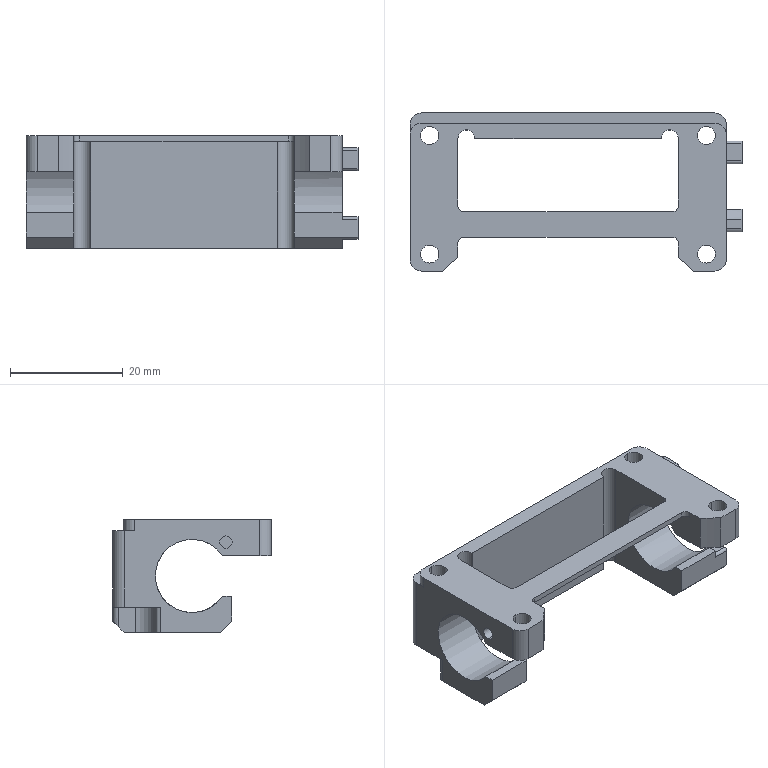NC program | Mastercam | posted with a generic post | part box 58.8 x 28 x 20 mm
Lines 21588 to 23685 of 29451, first 1908 of 2098 lines:
(3 FEM |TOOL - 3|DIA. OFF. - 3|LEN. - 3|TOOL DIA. - 3.)
N3638 T3 M6
N3640 G0 G54 G90 X19.135 Y5.752 C0. B0. S6000 M3
N3642 G43 H3 Z25.
N3644 Z1.
N3646 G1 Z-.25 F600.
N3648 X19.285 F2000.
N3650 G3 X19.435 Y5.902 J.15
N3652 G1 Y9.5
N3654 G2 X17.935 Y8. I-1.5
N3656 G1 X16.978
N3658 G3 X16.828 Y7.85 J-.15
N3660 G1 Y7.7
N3662 X19.135 Y5.752
N3664 Z-.5 F600.
N3666 X19.285 F2000.
N3668 G3 X19.435 Y5.902 J.15
N3670 G1 Y9.5
N3672 G2 X17.935 Y8. I-1.5
N3674 G1 X16.978
N3676 G3 X16.828 Y7.85 J-.15
N3678 G1 Y7.7
N3680 X19.135 Y5.752
N3682 Z-.75 F600.
N3684 X19.285 F2000.
N3686 G3 X19.435 Y5.902 J.15
N3688 G1 Y9.5
N3690 G2 X17.935 Y8. I-1.5
N3692 G1 X16.978
N3694 G3 X16.828 Y7.85 J-.15
N3696 G1 Y7.7
N3698 X19.135 Y5.752
N3700 Z-1. F600.
N3702 X19.285 F2000.
N3704 G3 X19.435 Y5.902 J.15
N3706 G1 Y9.5
N3708 G2 X17.935 Y8. I-1.5
N3710 G1 X16.978
N3712 G3 X16.828 Y7.85 J-.15
N3714 G1 Y7.7
N3716 X19.135 Y5.752
N3718 Z-1.25 F600.
N3720 X19.285 F2000.
N3722 G3 X19.435 Y5.902 J.15
N3724 G1 Y9.5
N3726 G2 X17.935 Y8. I-1.5
N3728 G1 X16.978
N3730 G3 X16.828 Y7.85 J-.15
N3732 G1 Y7.7
N3734 X19.135 Y5.752
N3736 Z-1.5 F600.
N3738 X19.285 F2000.
N3740 G3 X19.435 Y5.902 J.15
N3742 G1 Y9.5
N3744 G2 X17.935 Y8. I-1.5
N3746 G1 X16.978
N3748 G3 X16.828 Y7.85 J-.15
N3750 G1 Y7.7
N3752 X19.135 Y5.752
N3754 Z-1.75 F600.
N3756 X19.285 F2000.
N3758 G3 X19.435 Y5.902 J.15
N3760 G1 Y9.5
N3762 G2 X17.935 Y8. I-1.5
N3764 G1 X16.978
N3766 G3 X16.828 Y7.85 J-.15
N3768 G1 Y7.7
N3770 X19.135 Y5.752
N3772 Z-2. F600.
N3774 X19.285 F2000.
N3776 G3 X19.435 Y5.902 J.15
N3778 G1 Y9.5
N3780 G2 X17.935 Y8. I-1.5
N3782 G1 X16.978
N3784 G3 X16.828 Y7.85 J-.15
N3786 G1 Y7.7
N3788 X19.135 Y5.752
N3790 Z-2.25 F600.
N3792 X19.285 F2000.
N3794 G3 X19.435 Y5.902 J.15
N3796 G1 Y9.5
N3798 G2 X17.935 Y8. I-1.5
N3800 G1 X16.978
N3802 G3 X16.828 Y7.85 J-.15
N3804 G1 Y7.7
N3806 X19.135 Y5.752
N3808 Z-2.5 F600.
N3810 X19.285 F2000.
N3812 G3 X19.435 Y5.902 J.15
N3814 G1 Y9.5
N3816 G2 X17.935 Y8. I-1.5
N3818 G1 X16.978
N3820 G3 X16.828 Y7.85 J-.15
N3822 G1 Y7.7
N3824 X19.135 Y5.752
N3826 Z-2.75 F600.
N3828 X19.285 F2000.
N3830 G3 X19.435 Y5.902 J.15
N3832 G1 Y9.5
N3834 G2 X17.935 Y8. I-1.5
N3836 G1 X16.978
N3838 G3 X16.828 Y7.85 J-.15
N3840 G1 Y7.7
N3842 X19.135 Y5.752
N3844 Z-3. F600.
N3846 X19.285 F2000.
N3848 G3 X19.435 Y5.902 J.15
N3850 G1 Y9.5
N3852 G2 X17.935 Y8. I-1.5
N3854 G1 X16.978
N3856 G3 X16.828 Y7.85 J-.15
N3858 G1 Y7.7
N3860 X19.135 Y5.752
N3862 Z-3.25 F600.
N3864 X19.285 F2000.
N3866 G3 X19.435 Y5.902 J.15
N3868 G1 Y9.5
N3870 G2 X17.935 Y8. I-1.5
N3872 G1 X16.978
N3874 G3 X16.828 Y7.85 J-.15
N3876 G1 Y7.7
N3878 X19.135 Y5.752
N3880 Z-3.5 F600.
N3882 X19.285 F2000.
N3884 G3 X19.435 Y5.902 J.15
N3886 G1 Y9.5
N3888 G2 X17.935 Y8. I-1.5
N3890 G1 X16.978
N3892 G3 X16.828 Y7.85 J-.15
N3894 G1 Y7.7
N3896 X19.135 Y5.752
N3898 Z-3.75 F600.
N3900 X19.285 F2000.
N3902 G3 X19.435 Y5.902 J.15
N3904 G1 Y9.5
N3906 G2 X17.935 Y8. I-1.5
N3908 G1 X16.978
N3910 G3 X16.828 Y7.85 J-.15
N3912 G1 Y7.7
N3914 X19.135 Y5.752
N3916 Z-4. F600.
N3918 X19.285 F2000.
N3920 G3 X19.435 Y5.902 J.15
N3922 G1 Y9.5
N3924 G2 X17.935 Y8. I-1.5
N3926 G1 X16.978
N3928 G3 X16.828 Y7.85 J-.15
N3930 G1 Y7.7
N3932 X19.135 Y5.752
N3934 Z-4.25 F600.
N3936 X19.285 F2000.
N3938 G3 X19.435 Y5.902 J.15
N3940 G1 Y9.5
N3942 G2 X17.935 Y8. I-1.5
N3944 G1 X16.978
N3946 G3 X16.828 Y7.85 J-.15
N3948 G1 Y7.7
N3950 X19.135 Y5.752
N3952 Z-4.5 F600.
N3954 X19.285 F2000.
N3956 G3 X19.435 Y5.902 J.15
N3958 G1 Y9.5
N3960 G2 X17.935 Y8. I-1.5
N3962 G1 X16.978
N3964 G3 X16.828 Y7.85 J-.15
N3966 G1 Y7.7
N3968 X19.135 Y5.752
N3970 Z-4.75 F600.
N3972 X19.285 F2000.
N3974 G3 X19.435 Y5.902 J.15
N3976 G1 Y9.5
N3978 G2 X17.935 Y8. I-1.5
N3980 G1 X16.978
N3982 G3 X16.828 Y7.85 J-.15
N3984 G1 Y7.7
N3986 X19.135 Y5.752
N3988 Z-5. F600.
N3990 X19.285 F2000.
N3992 G3 X19.435 Y5.902 J.15
N3994 G1 Y9.5
N3996 G2 X17.935 Y8. I-1.5
N3998 G1 X16.978
N4000 G3 X16.828 Y7.85 J-.15
N4002 G1 Y7.7
N4004 X19.135 Y5.752
N4006 Z-5.25 F600.
N4008 X19.285 F2000.
N4010 G3 X19.435 Y5.902 J.15
N4012 G1 Y9.5
N4014 G2 X17.935 Y8. I-1.5
N4016 G1 X16.978
N4018 G3 X16.828 Y7.85 J-.15
N4020 G1 Y7.7
N4022 X19.135 Y5.752
N4024 Z-5.5 F600.
N4026 X19.285 F2000.
N4028 G3 X19.435 Y5.902 J.15
N4030 G1 Y9.5
N4032 G2 X17.935 Y8. I-1.5
N4034 G1 X16.978
N4036 G3 X16.828 Y7.85 J-.15
N4038 G1 Y7.7
N4040 X19.135 Y5.752
N4042 Z-5.75 F600.
N4044 X19.285 F2000.
N4046 G3 X19.435 Y5.902 J.15
N4048 G1 Y9.5
N4050 G2 X17.935 Y8. I-1.5
N4052 G1 X16.978
N4054 G3 X16.828 Y7.85 J-.15
N4056 G1 Y7.7
N4058 X19.135 Y5.752
N4060 Z-6. F600.
N4062 X19.285 F2000.
N4064 G3 X19.435 Y5.902 J.15
N4066 G1 Y9.5
N4068 G2 X17.935 Y8. I-1.5
N4070 G1 X16.978
N4072 G3 X16.828 Y7.85 J-.15
N4074 G1 Y7.7
N4076 X19.135 Y5.752
N4078 Z-6.25 F600.
N4080 X19.285 F2000.
N4082 G3 X19.435 Y5.902 J.15
N4084 G1 Y9.5
N4086 G2 X17.935 Y8. I-1.5
N4088 G1 X16.978
N4090 G3 X16.828 Y7.85 J-.15
N4092 G1 Y7.7
N4094 X19.135 Y5.752
N4096 Z-6.5 F600.
N4098 X19.285 F2000.
N4100 G3 X19.435 Y5.902 J.15
N4102 G1 Y9.5
N4104 G2 X17.935 Y8. I-1.5
N4106 G1 X16.978
N4108 G3 X16.828 Y7.85 J-.15
N4110 G1 Y7.7
N4112 X19.135 Y5.752
N4114 Z-6.75 F600.
N4116 X19.285 F2000.
N4118 G3 X19.435 Y5.902 J.15
N4120 G1 Y9.5
N4122 G2 X17.935 Y8. I-1.5
N4124 G1 X16.978
N4126 G3 X16.828 Y7.85 J-.15
N4128 G1 Y7.7
N4130 X19.135 Y5.752
N4132 Z-7. F600.
N4134 X19.285 F2000.
N4136 G3 X19.435 Y5.902 J.15
N4138 G1 Y9.5
N4140 G2 X17.935 Y8. I-1.5
N4142 G1 X16.978
N4144 G3 X16.828 Y7.85 J-.15
N4146 G1 Y7.7
N4148 X19.135 Y5.752
N4150 Z-7.25 F600.
N4152 X19.285 F2000.
N4154 G3 X19.435 Y5.902 J.15
N4156 G1 Y9.5
N4158 G2 X17.935 Y8. I-1.5
N4160 G1 X16.978
N4162 G3 X16.828 Y7.85 J-.15
N4164 G1 Y7.7
N4166 X19.135 Y5.752
N4168 Z-7.5 F600.
N4170 X19.285 F2000.
N4172 G3 X19.435 Y5.902 J.15
N4174 G1 Y9.5
N4176 G2 X17.935 Y8. I-1.5
N4178 G1 X16.978
N4180 G3 X16.828 Y7.85 J-.15
N4182 G1 Y7.7
N4184 X19.135 Y5.752
N4186 Z-7.75 F600.
N4188 X19.285 F2000.
N4190 G3 X19.435 Y5.902 J.15
N4192 G1 Y9.5
N4194 G2 X17.935 Y8. I-1.5
N4196 G1 X16.978
N4198 G3 X16.828 Y7.85 J-.15
N4200 G1 Y7.7
N4202 X19.135 Y5.752
N4204 Z-8. F600.
N4206 X19.285 F2000.
N4208 G3 X19.435 Y5.902 J.15
N4210 G1 Y9.5
N4212 G2 X17.935 Y8. I-1.5
N4214 G1 X16.978
N4216 G3 X16.828 Y7.85 J-.15
N4218 G1 Y7.7
N4220 X19.135 Y5.752
N4222 Z-8.25 F600.
N4224 X19.285 F2000.
N4226 G3 X19.435 Y5.902 J.15
N4228 G1 Y9.5
N4230 G2 X17.935 Y8. I-1.5
N4232 G1 X16.978
N4234 G3 X16.828 Y7.85 J-.15
N4236 G1 Y7.7
N4238 X19.135 Y5.752
N4240 Z-8.5 F600.
N4242 X19.285 F2000.
N4244 G3 X19.435 Y5.902 J.15
N4246 G1 Y9.5
N4248 G2 X17.935 Y8. I-1.5
N4250 G1 X16.978
N4252 G3 X16.828 Y7.85 J-.15
N4254 G1 Y7.7
N4256 X19.135 Y5.752
N4258 Z-8.75 F600.
N4260 X19.285 F2000.
N4262 G3 X19.435 Y5.902 J.15
N4264 G1 Y9.5
N4266 G2 X17.935 Y8. I-1.5
N4268 G1 X16.978
N4270 G3 X16.828 Y7.85 J-.15
N4272 G1 Y7.7
N4274 X19.135 Y5.752
N4276 Z-9. F600.
N4278 X19.285 F2000.
N4280 G3 X19.435 Y5.902 J.15
N4282 G1 Y9.5
N4284 G2 X17.935 Y8. I-1.5
N4286 G1 X16.978
N4288 G3 X16.828 Y7.85 J-.15
N4290 G1 Y7.7
N4292 X19.135 Y5.752
N4294 Z-9.25 F600.
N4296 X19.285 F2000.
N4298 G3 X19.435 Y5.902 J.15
N4300 G1 Y9.5
N4302 G2 X17.935 Y8. I-1.5
N4304 G1 X16.978
N4306 G3 X16.828 Y7.85 J-.15
N4308 G1 Y7.7
N4310 X19.135 Y5.752
N4312 Z-9.5 F600.
N4314 X19.285 F2000.
N4316 G3 X19.435 Y5.902 J.15
N4318 G1 Y9.5
N4320 G2 X17.935 Y8. I-1.5
N4322 G1 X16.978
N4324 G3 X16.828 Y7.85 J-.15
N4326 G1 Y7.7
N4328 X19.135 Y5.752
N4330 Z-9.75 F600.
N4332 X19.285 F2000.
N4334 G3 X19.435 Y5.902 J.15
N4336 G1 Y9.5
N4338 G2 X17.935 Y8. I-1.5
N4340 G1 X16.978
N4342 G3 X16.828 Y7.85 J-.15
N4344 G1 Y7.7
N4346 X19.135 Y5.752
N4348 Z-10. F600.
N4350 X19.285 F2000.
N4352 G3 X19.435 Y5.902 J.15
N4354 G1 Y9.5
N4356 G2 X17.935 Y8. I-1.5
N4358 G1 X16.978
N4360 G3 X16.828 Y7.85 J-.15
N4362 G1 Y7.7
N4364 X19.135 Y5.752
N4366 Z-10.25 F600.
N4368 X19.285 F2000.
N4370 G3 X19.435 Y5.902 J.15
N4372 G1 Y9.5
N4374 G2 X17.935 Y8. I-1.5
N4376 G1 X16.978
N4378 G3 X16.828 Y7.85 J-.15
N4380 G1 Y7.7
N4382 X19.135 Y5.752
N4384 Z-10.5 F600.
N4386 X19.285 F2000.
N4388 G3 X19.435 Y5.902 J.15
N4390 G1 Y9.5
N4392 G2 X17.935 Y8. I-1.5
N4394 G1 X16.978
N4396 G3 X16.828 Y7.85 J-.15
N4398 G1 Y7.7
N4400 X19.135 Y5.752
N4402 Z-10.75 F600.
N4404 X19.285 F2000.
N4406 G3 X19.435 Y5.902 J.15
N4408 G1 Y9.5
N4410 G2 X17.935 Y8. I-1.5
N4412 G1 X16.978
N4414 G3 X16.828 Y7.85 J-.15
N4416 G1 Y7.7
N4418 X19.135 Y5.752
N4420 Z-11. F600.
N4422 X19.285 F2000.
N4424 G3 X19.435 Y5.902 J.15
N4426 G1 Y9.5
N4428 G2 X17.935 Y8. I-1.5
N4430 G1 X16.978
N4432 G3 X16.828 Y7.85 J-.15
N4434 G1 Y7.7
N4436 X19.135 Y5.752
N4438 Z-11.25 F600.
N4440 X19.285 F2000.
N4442 G3 X19.435 Y5.902 J.15
N4444 G1 Y9.5
N4446 G2 X17.935 Y8. I-1.5
N4448 G1 X16.978
N4450 G3 X16.828 Y7.85 J-.15
N4452 G1 Y7.7
N4454 X19.135 Y5.752
N4456 Z-11.5 F600.
N4458 X19.285 F2000.
N4460 G3 X19.435 Y5.902 J.15
N4462 G1 Y9.5
N4464 G2 X17.935 Y8. I-1.5
N4466 G1 X16.978
N4468 G3 X16.828 Y7.85 J-.15
N4470 G1 Y7.7
N4472 X19.135 Y5.752
N4474 Z-11.75 F600.
N4476 X19.285 F2000.
N4478 G3 X19.435 Y5.902 J.15
N4480 G1 Y9.5
N4482 G2 X17.935 Y8. I-1.5
N4484 G1 X16.978
N4486 G3 X16.828 Y7.85 J-.15
N4488 G1 Y7.7
N4490 X19.135 Y5.752
N4492 Z-12. F600.
N4494 X19.285 F2000.
N4496 G3 X19.435 Y5.902 J.15
N4498 G1 Y9.5
N4500 G2 X17.935 Y8. I-1.5
N4502 G1 X16.978
N4504 G3 X16.828 Y7.85 J-.15
N4506 G1 Y7.7
N4508 X19.135 Y5.752
N4510 Z-12.25 F600.
N4512 X19.285 F2000.
N4514 G3 X19.435 Y5.902 J.15
N4516 G1 Y9.5
N4518 G2 X17.935 Y8. I-1.5
N4520 G1 X16.978
N4522 G3 X16.828 Y7.85 J-.15
N4524 G1 Y7.7
N4526 X19.135 Y5.752
N4528 Z-12.5 F600.
N4530 X19.285 F2000.
N4532 G3 X19.435 Y5.902 J.15
N4534 G1 Y9.5
N4536 G2 X17.935 Y8. I-1.5
N4538 G1 X16.978
N4540 G3 X16.828 Y7.85 J-.15
N4542 G1 Y7.7
N4544 X19.135 Y5.752
N4546 Z-12.75 F600.
N4548 X19.285 F2000.
N4550 G3 X19.435 Y5.902 J.15
N4552 G1 Y9.5
N4554 G2 X17.935 Y8. I-1.5
N4556 G1 X16.978
N4558 G3 X16.828 Y7.85 J-.15
N4560 G1 Y7.7
N4562 X19.135 Y5.752
N4564 Z-13. F600.
N4566 X19.285 F2000.
N4568 G3 X19.435 Y5.902 J.15
N4570 G1 Y9.5
N4572 G2 X17.935 Y8. I-1.5
N4574 G1 X16.978
N4576 G3 X16.828 Y7.85 J-.15
N4578 G1 Y7.7
N4580 X19.135 Y5.752
N4582 Z-13.25 F600.
N4584 X19.285 F2000.
N4586 G3 X19.435 Y5.902 J.15
N4588 G1 Y9.5
N4590 G2 X17.935 Y8. I-1.5
N4592 G1 X16.978
N4594 G3 X16.828 Y7.85 J-.15
N4596 G1 Y7.7
N4598 X19.135 Y5.752
N4600 Z-13.5 F600.
N4602 X19.285 F2000.
N4604 G3 X19.435 Y5.902 J.15
N4606 G1 Y9.5
N4608 G2 X17.935 Y8. I-1.5
N4610 G1 X16.978
N4612 G3 X16.828 Y7.85 J-.15
N4614 G1 Y7.7
N4616 X19.135 Y5.752
N4618 Z-13.75 F600.
N4620 X19.285 F2000.
N4622 G3 X19.435 Y5.902 J.15
N4624 G1 Y9.5
N4626 G2 X17.935 Y8. I-1.5
N4628 G1 X16.978
N4630 G3 X16.828 Y7.85 J-.15
N4632 G1 Y7.7
N4634 X19.135 Y5.752
N4636 Z-14. F600.
N4638 X19.285 F2000.
N4640 G3 X19.435 Y5.902 J.15
N4642 G1 Y9.5
N4644 G2 X17.935 Y8. I-1.5
N4646 G1 X16.978
N4648 G3 X16.828 Y7.85 J-.15
N4650 G1 Y7.7
N4652 X19.135 Y5.752
N4654 Z-14.25 F600.
N4656 X19.285 F2000.
N4658 G3 X19.435 Y5.902 J.15
N4660 G1 Y9.5
N4662 G2 X17.935 Y8. I-1.5
N4664 G1 X16.978
N4666 G3 X16.828 Y7.85 J-.15
N4668 G1 Y7.7
N4670 X19.135 Y5.752
N4672 Z-14.5 F600.
N4674 X19.285 F2000.
N4676 G3 X19.435 Y5.902 J.15
N4678 G1 Y9.5
N4680 G2 X17.935 Y8. I-1.5
N4682 G1 X16.978
N4684 G3 X16.828 Y7.85 J-.15
N4686 G1 Y7.7
N4688 X19.135 Y5.752
N4690 Z-14.75 F600.
N4692 X19.285 F2000.
N4694 G3 X19.435 Y5.902 J.15
N4696 G1 Y9.5
N4698 G2 X17.935 Y8. I-1.5
N4700 G1 X16.978
N4702 G3 X16.828 Y7.85 J-.15
N4704 G1 Y7.7
N4706 X19.135 Y5.752
N4708 Z-15. F600.
N4710 X19.285 F2000.
N4712 G3 X19.435 Y5.902 J.15
N4714 G1 Y9.5
N4716 G2 X17.935 Y8. I-1.5
N4718 G1 X16.978
N4720 G3 X16.828 Y7.85 J-.15
N4722 G1 Y7.7
N4724 X19.135 Y5.752
N4726 Z-15.25 F600.
N4728 X19.285 F2000.
N4730 G3 X19.435 Y5.902 J.15
N4732 G1 Y9.5
N4734 G2 X17.935 Y8. I-1.5
N4736 G1 X16.978
N4738 G3 X16.828 Y7.85 J-.15
N4740 G1 Y7.7
N4742 X19.135 Y5.752
N4744 Z-15.5 F600.
N4746 X19.285 F2000.
N4748 G3 X19.435 Y5.902 J.15
N4750 G1 Y9.5
N4752 G2 X17.935 Y8. I-1.5
N4754 G1 X16.978
N4756 G3 X16.828 Y7.85 J-.15
N4758 G1 Y7.7
N4760 X19.135 Y5.752
N4762 Z-15.75 F600.
N4764 X19.285 F2000.
N4766 G3 X19.435 Y5.902 J.15
N4768 G1 Y9.5
N4770 G2 X17.935 Y8. I-1.5
N4772 G1 X16.978
N4774 G3 X16.828 Y7.85 J-.15
N4776 G1 Y7.7
N4778 X19.135 Y5.752
N4780 Z-16. F600.
N4782 X19.285 F2000.
N4784 G3 X19.435 Y5.902 J.15
N4786 G1 Y9.5
N4788 G2 X17.935 Y8. I-1.5
N4790 G1 X16.978
N4792 G3 X16.828 Y7.85 J-.15
N4794 G1 Y7.7
N4796 X19.135 Y5.752
N4798 Z-16.25 F600.
N4800 X19.285 F2000.
N4802 G3 X19.435 Y5.902 J.15
N4804 G1 Y9.5
N4806 G2 X17.935 Y8. I-1.5
N4808 G1 X16.978
N4810 G3 X16.828 Y7.85 J-.15
N4812 G1 Y7.7
N4814 X19.135 Y5.752
N4816 Z-16.5 F600.
N4818 X19.285 F2000.
N4820 G3 X19.435 Y5.902 J.15
N4822 G1 Y9.5
N4824 G2 X17.935 Y8. I-1.5
N4826 G1 X16.978
N4828 G3 X16.828 Y7.85 J-.15
N4830 G1 Y7.7
N4832 X19.135 Y5.752
N4834 Z-16.75 F600.
N4836 X19.285 F2000.
N4838 G3 X19.435 Y5.902 J.15
N4840 G1 Y9.5
N4842 G2 X17.935 Y8. I-1.5
N4844 G1 X16.978
N4846 G3 X16.828 Y7.85 J-.15
N4848 G1 Y7.7
N4850 X19.135 Y5.752
N4852 Z-17. F600.
N4854 X19.285 F2000.
N4856 G3 X19.435 Y5.902 J.15
N4858 G1 Y9.5
N4860 G2 X17.935 Y8. I-1.5
N4862 G1 X16.978
N4864 G3 X16.828 Y7.85 J-.15
N4866 G1 Y7.7
N4868 X19.135 Y5.752
N4870 Z-17.25 F600.
N4872 X19.285 F2000.
N4874 G3 X19.435 Y5.902 J.15
N4876 G1 Y9.5
N4878 G2 X17.935 Y8. I-1.5
N4880 G1 X16.978
N4882 G3 X16.828 Y7.85 J-.15
N4884 G1 Y7.7
N4886 X19.135 Y5.752
N4888 Z-17.5 F600.
N4890 X19.285 F2000.
N4892 G3 X19.435 Y5.902 J.15
N4894 G1 Y9.5
N4896 G2 X17.935 Y8. I-1.5
N4898 G1 X16.978
N4900 G3 X16.828 Y7.85 J-.15
N4902 G1 Y7.7
N4904 X19.135 Y5.752
N4906 Z-17.75 F600.
N4908 X19.285 F2000.
N4910 G3 X19.435 Y5.902 J.15
N4912 G1 Y9.5
N4914 G2 X17.935 Y8. I-1.5
N4916 G1 X16.978
N4918 G3 X16.828 Y7.85 J-.15
N4920 G1 Y7.7
N4922 X19.135 Y5.752
N4924 Z-18. F600.
N4926 X19.285 F2000.
N4928 G3 X19.435 Y5.902 J.15
N4930 G1 Y9.5
N4932 G2 X17.935 Y8. I-1.5
N4934 G1 X16.978
N4936 G3 X16.828 Y7.85 J-.15
N4938 G1 Y7.7
N4940 X19.135 Y5.752
N4942 Z-18.25 F600.
N4944 X19.285 F2000.
N4946 G3 X19.435 Y5.902 J.15
N4948 G1 Y9.5
N4950 G2 X17.935 Y8. I-1.5
N4952 G1 X16.978
N4954 G3 X16.828 Y7.85 J-.15
N4956 G1 Y7.7
N4958 X19.135 Y5.752
N4960 Z-18.5 F600.
N4962 X19.285 F2000.
N4964 G3 X19.435 Y5.902 J.15
N4966 G1 Y9.5
N4968 G2 X17.935 Y8. I-1.5
N4970 G1 X16.978
N4972 G3 X16.828 Y7.85 J-.15
N4974 G1 Y7.7
N4976 X19.135 Y5.752
N4978 Z-18.75 F600.
N4980 X19.285 F2000.
N4982 G3 X19.435 Y5.902 J.15
N4984 G1 Y9.5
N4986 G2 X17.935 Y8. I-1.5
N4988 G1 X16.978
N4990 G3 X16.828 Y7.85 J-.15
N4992 G1 Y7.7
N4994 X19.135 Y5.752
N4996 Z-19. F600.
N4998 X19.285 F2000.
N5000 G3 X19.435 Y5.902 J.15
N5002 G1 Y9.5
N5004 G2 X17.935 Y8. I-1.5
N5006 G1 X16.978
N5008 G3 X16.828 Y7.85 J-.15
N5010 G1 Y7.7
N5012 X19.135 Y5.752
N5014 Z-19.25 F600.
N5016 X19.285 F2000.
N5018 G3 X19.435 Y5.902 J.15
N5020 G1 Y9.5
N5022 G2 X17.935 Y8. I-1.5
N5024 G1 X16.978
N5026 G3 X16.828 Y7.85 J-.15
N5028 G1 Y7.7
N5030 X19.135 Y5.752
N5032 Z-19.5 F600.
N5034 X19.285 F2000.
N5036 G3 X19.435 Y5.902 J.15
N5038 G1 Y9.5
N5040 G2 X17.935 Y8. I-1.5
N5042 G1 X16.978
N5044 G3 X16.828 Y7.85 J-.15
N5046 G1 Y7.7
N5048 X19.135 Y5.752
N5050 Z-19.75 F600.
N5052 X19.285 F2000.
N5054 G3 X19.435 Y5.902 J.15
N5056 G1 Y9.5
N5058 G2 X17.935 Y8. I-1.5
N5060 G1 X16.978
N5062 G3 X16.828 Y7.85 J-.15
N5064 G1 Y7.7
N5066 X19.135 Y5.752
N5068 Z-20. F600.
N5070 X19.285 F2000.
N5072 G3 X19.435 Y5.902 J.15
N5074 G1 Y9.5
N5076 G2 X17.935 Y8. I-1.5
N5078 G1 X16.978
N5080 G3 X16.828 Y7.85 J-.15
N5082 G1 Y7.7
N5084 X19.135 Y5.752
N5086 Z-20.25 F600.
N5088 X19.285 F2000.
N5090 G3 X19.435 Y5.902 J.15
N5092 G1 Y9.5
N5094 G2 X17.935 Y8. I-1.5
N5096 G1 X16.978
N5098 G3 X16.828 Y7.85 J-.15
N5100 G1 Y7.7
N5102 X19.135 Y5.752
N5104 Z-20.5 F600.
N5106 X19.285 F2000.
N5108 G3 X19.435 Y5.902 J.15
N5110 G1 Y9.5
N5112 G2 X17.935 Y8. I-1.5
N5114 G1 X16.978
N5116 G3 X16.828 Y7.85 J-.15
N5118 G1 Y7.7
N5120 G0 Z25.
N5122 X-14.028
N5124 Z1.
N5126 G1 Z-.25 F600.
N5128 Y7.85 F2000.
N5130 G3 X-14.178 Y8. I-.15
N5132 G1 X-15.135
N5134 G2 X-16.635 Y9.5 J1.5
N5136 G1 Y5.902
N5138 G3 X-16.485 Y5.752 I.15
N5140 G1 X-16.335
N5142 X-14.028 Y7.7
N5144 Z-.5 F600.
N5146 Y7.85 F2000.
N5148 G3 X-14.178 Y8. I-.15
N5150 G1 X-15.135
N5152 G2 X-16.635 Y9.5 J1.5
N5154 G1 Y5.902
N5156 G3 X-16.485 Y5.752 I.15
N5158 G1 X-16.335
N5160 X-14.028 Y7.7
N5162 Z-.75 F600.
N5164 Y7.85 F2000.
N5166 G3 X-14.178 Y8. I-.15
N5168 G1 X-15.135
N5170 G2 X-16.635 Y9.5 J1.5
N5172 G1 Y5.902
N5174 G3 X-16.485 Y5.752 I.15
N5176 G1 X-16.335
N5178 X-14.028 Y7.7
N5180 Z-1. F600.
N5182 Y7.85 F2000.
N5184 G3 X-14.178 Y8. I-.15
N5186 G1 X-15.135
N5188 G2 X-16.635 Y9.5 J1.5
N5190 G1 Y5.902
N5192 G3 X-16.485 Y5.752 I.15
N5194 G1 X-16.335
N5196 X-14.028 Y7.7
N5198 Z-1.25 F600.
N5200 Y7.85 F2000.
N5202 G3 X-14.178 Y8. I-.15
N5204 G1 X-15.135
N5206 G2 X-16.635 Y9.5 J1.5
N5208 G1 Y5.902
N5210 G3 X-16.485 Y5.752 I.15
N5212 G1 X-16.335
N5214 X-14.028 Y7.7
N5216 Z-1.5 F600.
N5218 Y7.85 F2000.
N5220 G3 X-14.178 Y8. I-.15
N5222 G1 X-15.135
N5224 G2 X-16.635 Y9.5 J1.5
N5226 G1 Y5.902
N5228 G3 X-16.485 Y5.752 I.15
N5230 G1 X-16.335
N5232 X-14.028 Y7.7
N5234 Z-1.75 F600.
N5236 Y7.85 F2000.
N5238 G3 X-14.178 Y8. I-.15
N5240 G1 X-15.135
N5242 G2 X-16.635 Y9.5 J1.5
N5244 G1 Y5.902
N5246 G3 X-16.485 Y5.752 I.15
N5248 G1 X-16.335
N5250 X-14.028 Y7.7
N5252 Z-2. F600.
N5254 Y7.85 F2000.
N5256 G3 X-14.178 Y8. I-.15
N5258 G1 X-15.135
N5260 G2 X-16.635 Y9.5 J1.5
N5262 G1 Y5.902
N5264 G3 X-16.485 Y5.752 I.15
N5266 G1 X-16.335
N5268 X-14.028 Y7.7
N5270 Z-2.25 F600.
N5272 Y7.85 F2000.
N5274 G3 X-14.178 Y8. I-.15
N5276 G1 X-15.135
N5278 G2 X-16.635 Y9.5 J1.5
N5280 G1 Y5.902
N5282 G3 X-16.485 Y5.752 I.15
N5284 G1 X-16.335
N5286 X-14.028 Y7.7
N5288 Z-2.5 F600.
N5290 Y7.85 F2000.
N5292 G3 X-14.178 Y8. I-.15
N5294 G1 X-15.135
N5296 G2 X-16.635 Y9.5 J1.5
N5298 G1 Y5.902
N5300 G3 X-16.485 Y5.752 I.15
N5302 G1 X-16.335
N5304 X-14.028 Y7.7
N5306 Z-2.75 F600.
N5308 Y7.85 F2000.
N5310 G3 X-14.178 Y8. I-.15
N5312 G1 X-15.135
N5314 G2 X-16.635 Y9.5 J1.5
N5316 G1 Y5.902
N5318 G3 X-16.485 Y5.752 I.15
N5320 G1 X-16.335
N5322 X-14.028 Y7.7
N5324 Z-3. F600.
N5326 Y7.85 F2000.
N5328 G3 X-14.178 Y8. I-.15
N5330 G1 X-15.135
N5332 G2 X-16.635 Y9.5 J1.5
N5334 G1 Y5.902
N5336 G3 X-16.485 Y5.752 I.15
N5338 G1 X-16.335
N5340 X-14.028 Y7.7
N5342 Z-3.25 F600.
N5344 Y7.85 F2000.
N5346 G3 X-14.178 Y8. I-.15
N5348 G1 X-15.135
N5350 G2 X-16.635 Y9.5 J1.5
N5352 G1 Y5.902
N5354 G3 X-16.485 Y5.752 I.15
N5356 G1 X-16.335
N5358 X-14.028 Y7.7
N5360 Z-3.5 F600.
N5362 Y7.85 F2000.
N5364 G3 X-14.178 Y8. I-.15
N5366 G1 X-15.135
N5368 G2 X-16.635 Y9.5 J1.5
N5370 G1 Y5.902
N5372 G3 X-16.485 Y5.752 I.15
N5374 G1 X-16.335
N5376 X-14.028 Y7.7
N5378 Z-3.75 F600.
N5380 Y7.85 F2000.
N5382 G3 X-14.178 Y8. I-.15
N5384 G1 X-15.135
N5386 G2 X-16.635 Y9.5 J1.5
N5388 G1 Y5.902
N5390 G3 X-16.485 Y5.752 I.15
N5392 G1 X-16.335
N5394 X-14.028 Y7.7
N5396 Z-4. F600.
N5398 Y7.85 F2000.
N5400 G3 X-14.178 Y8. I-.15
N5402 G1 X-15.135
N5404 G2 X-16.635 Y9.5 J1.5
N5406 G1 Y5.902
N5408 G3 X-16.485 Y5.752 I.15
N5410 G1 X-16.335
N5412 X-14.028 Y7.7
N5414 Z-4.25 F600.
N5416 Y7.85 F2000.
N5418 G3 X-14.178 Y8. I-.15
N5420 G1 X-15.135
N5422 G2 X-16.635 Y9.5 J1.5
N5424 G1 Y5.902
N5426 G3 X-16.485 Y5.752 I.15
N5428 G1 X-16.335
N5430 X-14.028 Y7.7
N5432 Z-4.5 F600.
N5434 Y7.85 F2000.
N5436 G3 X-14.178 Y8. I-.15
N5438 G1 X-15.135
N5440 G2 X-16.635 Y9.5 J1.5
N5442 G1 Y5.902
N5444 G3 X-16.485 Y5.752 I.15
N5446 G1 X-16.335
N5448 X-14.028 Y7.7
N5450 Z-4.75 F600.
N5452 Y7.85 F2000.
N5454 G3 X-14.178 Y8. I-.15
N5456 G1 X-15.135
N5458 G2 X-16.635 Y9.5 J1.5
N5460 G1 Y5.902
N5462 G3 X-16.485 Y5.752 I.15
N5464 G1 X-16.335
N5466 X-14.028 Y7.7
N5468 Z-5. F600.
N5470 Y7.85 F2000.
N5472 G3 X-14.178 Y8. I-.15
N5474 G1 X-15.135
N5476 G2 X-16.635 Y9.5 J1.5
N5478 G1 Y5.902
N5480 G3 X-16.485 Y5.752 I.15
N5482 G1 X-16.335
N5484 X-14.028 Y7.7
N5486 Z-5.25 F600.
N5488 Y7.85 F2000.
N5490 G3 X-14.178 Y8. I-.15
N5492 G1 X-15.135
N5494 G2 X-16.635 Y9.5 J1.5
N5496 G1 Y5.902
N5498 G3 X-16.485 Y5.752 I.15
N5500 G1 X-16.335
N5502 X-14.028 Y7.7
N5504 Z-5.5 F600.
N5506 Y7.85 F2000.
N5508 G3 X-14.178 Y8. I-.15
N5510 G1 X-15.135
N5512 G2 X-16.635 Y9.5 J1.5
N5514 G1 Y5.902
N5516 G3 X-16.485 Y5.752 I.15
N5518 G1 X-16.335
N5520 X-14.028 Y7.7
N5522 Z-5.75 F600.
N5524 Y7.85 F2000.
N5526 G3 X-14.178 Y8. I-.15
N5528 G1 X-15.135
N5530 G2 X-16.635 Y9.5 J1.5
N5532 G1 Y5.902
N5534 G3 X-16.485 Y5.752 I.15
N5536 G1 X-16.335
N5538 X-14.028 Y7.7
N5540 Z-6. F600.
N5542 Y7.85 F2000.
N5544 G3 X-14.178 Y8. I-.15
N5546 G1 X-15.135
N5548 G2 X-16.635 Y9.5 J1.5
N5550 G1 Y5.902
N5552 G3 X-16.485 Y5.752 I.15
N5554 G1 X-16.335
N5556 X-14.028 Y7.7
N5558 Z-6.25 F600.
N5560 Y7.85 F2000.
N5562 G3 X-14.178 Y8. I-.15
N5564 G1 X-15.135
N5566 G2 X-16.635 Y9.5 J1.5
N5568 G1 Y5.902
N5570 G3 X-16.485 Y5.752 I.15
N5572 G1 X-16.335
N5574 X-14.028 Y7.7
N5576 Z-6.5 F600.
N5578 Y7.85 F2000.
N5580 G3 X-14.178 Y8. I-.15
N5582 G1 X-15.135
N5584 G2 X-16.635 Y9.5 J1.5
N5586 G1 Y5.902
N5588 G3 X-16.485 Y5.752 I.15
N5590 G1 X-16.335
N5592 X-14.028 Y7.7
N5594 Z-6.75 F600.
N5596 Y7.85 F2000.
N5598 G3 X-14.178 Y8. I-.15
N5600 G1 X-15.135
N5602 G2 X-16.635 Y9.5 J1.5
N5604 G1 Y5.902
N5606 G3 X-16.485 Y5.752 I.15
N5608 G1 X-16.335
N5610 X-14.028 Y7.7
N5612 Z-7. F600.
N5614 Y7.85 F2000.
N5616 G3 X-14.178 Y8. I-.15
N5618 G1 X-15.135
N5620 G2 X-16.635 Y9.5 J1.5
N5622 G1 Y5.902
N5624 G3 X-16.485 Y5.752 I.15
N5626 G1 X-16.335
N5628 X-14.028 Y7.7
N5630 Z-7.25 F600.
N5632 Y7.85 F2000.
N5634 G3 X-14.178 Y8. I-.15
N5636 G1 X-15.135
N5638 G2 X-16.635 Y9.5 J1.5
N5640 G1 Y5.902
N5642 G3 X-16.485 Y5.752 I.15
N5644 G1 X-16.335
N5646 X-14.028 Y7.7
N5648 Z-7.5 F600.
N5650 Y7.85 F2000.
N5652 G3 X-14.178 Y8. I-.15
N5654 G1 X-15.135
N5656 G2 X-16.635 Y9.5 J1.5
N5658 G1 Y5.902
N5660 G3 X-16.485 Y5.752 I.15
N5662 G1 X-16.335
N5664 X-14.028 Y7.7
N5666 Z-7.75 F600.
N5668 Y7.85 F2000.
N5670 G3 X-14.178 Y8. I-.15
N5672 G1 X-15.135
N5674 G2 X-16.635 Y9.5 J1.5
N5676 G1 Y5.902
N5678 G3 X-16.485 Y5.752 I.15
N5680 G1 X-16.335
N5682 X-14.028 Y7.7
N5684 Z-8. F600.
N5686 Y7.85 F2000.
N5688 G3 X-14.178 Y8. I-.15
N5690 G1 X-15.135
N5692 G2 X-16.635 Y9.5 J1.5
N5694 G1 Y5.902
N5696 G3 X-16.485 Y5.752 I.15
N5698 G1 X-16.335
N5700 X-14.028 Y7.7
N5702 Z-8.25 F600.
N5704 Y7.85 F2000.
N5706 G3 X-14.178 Y8. I-.15
N5708 G1 X-15.135
N5710 G2 X-16.635 Y9.5 J1.5
N5712 G1 Y5.902
N5714 G3 X-16.485 Y5.752 I.15
N5716 G1 X-16.335
N5718 X-14.028 Y7.7
N5720 Z-8.5 F600.
N5722 Y7.85 F2000.
N5724 G3 X-14.178 Y8. I-.15
N5726 G1 X-15.135
N5728 G2 X-16.635 Y9.5 J1.5
N5730 G1 Y5.902
N5732 G3 X-16.485 Y5.752 I.15
N5734 G1 X-16.335
N5736 X-14.028 Y7.7
N5738 Z-8.75 F600.
N5740 Y7.85 F2000.
N5742 G3 X-14.178 Y8. I-.15
N5744 G1 X-15.135
N5746 G2 X-16.635 Y9.5 J1.5
N5748 G1 Y5.902
N5750 G3 X-16.485 Y5.752 I.15
N5752 G1 X-16.335
N5754 X-14.028 Y7.7
N5756 Z-9. F600.
N5758 Y7.85 F2000.
N5760 G3 X-14.178 Y8. I-.15
N5762 G1 X-15.135
N5764 G2 X-16.635 Y9.5 J1.5
N5766 G1 Y5.902
N5768 G3 X-16.485 Y5.752 I.15
N5770 G1 X-16.335
N5772 X-14.028 Y7.7
N5774 Z-9.25 F600.
N5776 Y7.85 F2000.
N5778 G3 X-14.178 Y8. I-.15
N5780 G1 X-15.135
N5782 G2 X-16.635 Y9.5 J1.5
N5784 G1 Y5.902
N5786 G3 X-16.485 Y5.752 I.15
N5788 G1 X-16.335
N5790 X-14.028 Y7.7
N5792 Z-9.5 F600.
N5794 Y7.85 F2000.
N5796 G3 X-14.178 Y8. I-.15
N5798 G1 X-15.135
N5800 G2 X-16.635 Y9.5 J1.5
N5802 G1 Y5.902
N5804 G3 X-16.485 Y5.752 I.15
N5806 G1 X-16.335
N5808 X-14.028 Y7.7
N5810 Z-9.75 F600.
N5812 Y7.85 F2000.
N5814 G3 X-14.178 Y8. I-.15
N5816 G1 X-15.135
N5818 G2 X-16.635 Y9.5 J1.5
N5820 G1 Y5.902
N5822 G3 X-16.485 Y5.752 I.15
N5824 G1 X-16.335
N5826 X-14.028 Y7.7
N5828 Z-10. F600.
N5830 Y7.85 F2000.
N5832 G3 X-14.178 Y8. I-.15
N5834 G1 X-15.135
N5836 G2 X-16.635 Y9.5 J1.5
N5838 G1 Y5.902
N5840 G3 X-16.485 Y5.752 I.15
N5842 G1 X-16.335
N5844 X-14.028 Y7.7
N5846 Z-10.25 F600.
N5848 Y7.85 F2000.
N5850 G3 X-14.178 Y8. I-.15
N5852 G1 X-15.135
N5854 G2 X-16.635 Y9.5 J1.5
N5856 G1 Y5.902
N5858 G3 X-16.485 Y5.752 I.15
N5860 G1 X-16.335
N5862 X-14.028 Y7.7
N5864 Z-10.5 F600.
N5866 Y7.85 F2000.
N5868 G3 X-14.178 Y8. I-.15
N5870 G1 X-15.135
N5872 G2 X-16.635 Y9.5 J1.5
N5874 G1 Y5.902
N5876 G3 X-16.485 Y5.752 I.15
N5878 G1 X-16.335
N5880 X-14.028 Y7.7
N5882 Z-10.75 F600.
N5884 Y7.85 F2000.
N5886 G3 X-14.178 Y8. I-.15
N5888 G1 X-15.135
N5890 G2 X-16.635 Y9.5 J1.5
N5892 G1 Y5.902
N5894 G3 X-16.485 Y5.752 I.15
N5896 G1 X-16.335
N5898 X-14.028 Y7.7
N5900 Z-11. F600.
N5902 Y7.85 F2000.
N5904 G3 X-14.178 Y8. I-.15
N5906 G1 X-15.135
N5908 G2 X-16.635 Y9.5 J1.5
N5910 G1 Y5.902
N5912 G3 X-16.485 Y5.752 I.15
N5914 G1 X-16.335
N5916 X-14.028 Y7.7
N5918 Z-11.25 F600.
N5920 Y7.85 F2000.
N5922 G3 X-14.178 Y8. I-.15
N5924 G1 X-15.135
N5926 G2 X-16.635 Y9.5 J1.5
N5928 G1 Y5.902
N5930 G3 X-16.485 Y5.752 I.15
N5932 G1 X-16.335
N5934 X-14.028 Y7.7
N5936 Z-11.5 F600.
N5938 Y7.85 F2000.
N5940 G3 X-14.178 Y8. I-.15
N5942 G1 X-15.135
N5944 G2 X-16.635 Y9.5 J1.5
N5946 G1 Y5.902
N5948 G3 X-16.485 Y5.752 I.15
N5950 G1 X-16.335
N5952 X-14.028 Y7.7
N5954 Z-11.75 F600.
N5956 Y7.85 F2000.
N5958 G3 X-14.178 Y8. I-.15
N5960 G1 X-15.135
N5962 G2 X-16.635 Y9.5 J1.5
N5964 G1 Y5.902
N5966 G3 X-16.485 Y5.752 I.15
N5968 G1 X-16.335
N5970 X-14.028 Y7.7
N5972 Z-12. F600.
N5974 Y7.85 F2000.
N5976 G3 X-14.178 Y8. I-.15
N5978 G1 X-15.135
N5980 G2 X-16.635 Y9.5 J1.5
N5982 G1 Y5.902
N5984 G3 X-16.485 Y5.752 I.15
N5986 G1 X-16.335
N5988 X-14.028 Y7.7
N5990 Z-12.25 F600.
N5992 Y7.85 F2000.
N5994 G3 X-14.178 Y8. I-.15
N5996 G1 X-15.135
N5998 G2 X-16.635 Y9.5 J1.5
N6000 G1 Y5.902
N6002 G3 X-16.485 Y5.752 I.15
N6004 G1 X-16.335
N6006 X-14.028 Y7.7
N6008 Z-12.5 F600.
N6010 Y7.85 F2000.
N6012 G3 X-14.178 Y8. I-.15
N6014 G1 X-15.135
N6016 G2 X-16.635 Y9.5 J1.5
N6018 G1 Y5.902
N6020 G3 X-16.485 Y5.752 I.15
N6022 G1 X-16.335
N6024 X-14.028 Y7.7
N6026 Z-12.75 F600.
N6028 Y7.85 F2000.
N6030 G3 X-14.178 Y8. I-.15
N6032 G1 X-15.135
N6034 G2 X-16.635 Y9.5 J1.5
N6036 G1 Y5.902
N6038 G3 X-16.485 Y5.752 I.15
N6040 G1 X-16.335
N6042 X-14.028 Y7.7
N6044 Z-13. F600.
N6046 Y7.85 F2000.
N6048 G3 X-14.178 Y8. I-.15
N6050 G1 X-15.135
N6052 G2 X-16.635 Y9.5 J1.5
N6054 G1 Y5.902
N6056 G3 X-16.485 Y5.752 I.15
N6058 G1 X-16.335
N6060 X-14.028 Y7.7
N6062 Z-13.25 F600.
N6064 Y7.85 F2000.
N6066 G3 X-14.178 Y8. I-.15
N6068 G1 X-15.135
N6070 G2 X-16.635 Y9.5 J1.5
N6072 G1 Y5.902
N6074 G3 X-16.485 Y5.752 I.15
N6076 G1 X-16.335
N6078 X-14.028 Y7.7
N6080 Z-13.5 F600.
N6082 Y7.85 F2000.
N6084 G3 X-14.178 Y8. I-.15
N6086 G1 X-15.135
N6088 G2 X-16.635 Y9.5 J1.5
N6090 G1 Y5.902
N6092 G3 X-16.485 Y5.752 I.15
N6094 G1 X-16.335
N6096 X-14.028 Y7.7
N6098 Z-13.75 F600.
N6100 Y7.85 F2000.
N6102 G3 X-14.178 Y8. I-.15
N6104 G1 X-15.135
N6106 G2 X-16.635 Y9.5 J1.5
N6108 G1 Y5.902
N6110 G3 X-16.485 Y5.752 I.15
N6112 G1 X-16.335
N6114 X-14.028 Y7.7
N6116 Z-14. F600.
N6118 Y7.85 F2000.
N6120 G3 X-14.178 Y8. I-.15
N6122 G1 X-15.135
N6124 G2 X-16.635 Y9.5 J1.5
N6126 G1 Y5.902
N6128 G3 X-16.485 Y5.752 I.15
N6130 G1 X-16.335
N6132 X-14.028 Y7.7
N6134 Z-14.25 F600.
N6136 Y7.85 F2000.
N6138 G3 X-14.178 Y8. I-.15
N6140 G1 X-15.135
N6142 G2 X-16.635 Y9.5 J1.5
N6144 G1 Y5.902
N6146 G3 X-16.485 Y5.752 I.15
N6148 G1 X-16.335
N6150 X-14.028 Y7.7
N6152 Z-14.5 F600.
N6154 Y7.85 F2000.
N6156 G3 X-14.178 Y8. I-.15
N6158 G1 X-15.135
N6160 G2 X-16.635 Y9.5 J1.5
N6162 G1 Y5.902
N6164 G3 X-16.485 Y5.752 I.15
N6166 G1 X-16.335
N6168 X-14.028 Y7.7
N6170 Z-14.75 F600.
N6172 Y7.85 F2000.
N6174 G3 X-14.178 Y8. I-.15
N6176 G1 X-15.135
N6178 G2 X-16.635 Y9.5 J1.5
N6180 G1 Y5.902
N6182 G3 X-16.485 Y5.752 I.15
N6184 G1 X-16.335
N6186 X-14.028 Y7.7
N6188 Z-15. F600.
N6190 Y7.85 F2000.
N6192 G3 X-14.178 Y8. I-.15
N6194 G1 X-15.135
N6196 G2 X-16.635 Y9.5 J1.5
N6198 G1 Y5.902
N6200 G3 X-16.485 Y5.752 I.15
N6202 G1 X-16.335
N6204 X-14.028 Y7.7
N6206 Z-15.25 F600.
N6208 Y7.85 F2000.
N6210 G3 X-14.178 Y8. I-.15
N6212 G1 X-15.135
N6214 G2 X-16.635 Y9.5 J1.5
N6216 G1 Y5.902
N6218 G3 X-16.485 Y5.752 I.15
N6220 G1 X-16.335
N6222 X-14.028 Y7.7
N6224 Z-15.5 F600.
N6226 Y7.85 F2000.
N6228 G3 X-14.178 Y8. I-.15
N6230 G1 X-15.135
N6232 G2 X-16.635 Y9.5 J1.5
N6234 G1 Y5.902
N6236 G3 X-16.485 Y5.752 I.15
N6238 G1 X-16.335
N6240 X-14.028 Y7.7
N6242 Z-15.75 F600.
N6244 Y7.85 F2000.
N6246 G3 X-14.178 Y8. I-.15
N6248 G1 X-15.135
N6250 G2 X-16.635 Y9.5 J1.5
N6252 G1 Y5.902
N6254 G3 X-16.485 Y5.752 I.15
N6256 G1 X-16.335
N6258 X-14.028 Y7.7
N6260 Z-16. F600.
N6262 Y7.85 F2000.
N6264 G3 X-14.178 Y8. I-.15
N6266 G1 X-15.135
N6268 G2 X-16.635 Y9.5 J1.5
N6270 G1 Y5.902
N6272 G3 X-16.485 Y5.752 I.15
N6274 G1 X-16.335
N6276 X-14.028 Y7.7
N6278 Z-16.25 F600.
N6280 Y7.85 F2000.
N6282 G3 X-14.178 Y8. I-.15
N6284 G1 X-15.135
N6286 G2 X-16.635 Y9.5 J1.5
N6288 G1 Y5.902
N6290 G3 X-16.485 Y5.752 I.15
N6292 G1 X-16.335
N6294 X-14.028 Y7.7
N6296 Z-16.5 F600.
N6298 Y7.85 F2000.
N6300 G3 X-14.178 Y8. I-.15
N6302 G1 X-15.135
N6304 G2 X-16.635 Y9.5 J1.5
N6306 G1 Y5.902
N6308 G3 X-16.485 Y5.752 I.15
N6310 G1 X-16.335
N6312 X-14.028 Y7.7
N6314 Z-16.75 F600.
N6316 Y7.85 F2000.
N6318 G3 X-14.178 Y8. I-.15
N6320 G1 X-15.135
N6322 G2 X-16.635 Y9.5 J1.5
N6324 G1 Y5.902
N6326 G3 X-16.485 Y5.752 I.15
N6328 G1 X-16.335
N6330 X-14.028 Y7.7
N6332 Z-17. F600.
N6334 Y7.85 F2000.
N6336 G3 X-14.178 Y8. I-.15
N6338 G1 X-15.135
N6340 G2 X-16.635 Y9.5 J1.5
N6342 G1 Y5.902
N6344 G3 X-16.485 Y5.752 I.15
N6346 G1 X-16.335
N6348 X-14.028 Y7.7
N6350 Z-17.25 F600.
N6352 Y7.85 F2000.
N6354 G3 X-14.178 Y8. I-.15
N6356 G1 X-15.135
N6358 G2 X-16.635 Y9.5 J1.5
N6360 G1 Y5.902
N6362 G3 X-16.485 Y5.752 I.15
N6364 G1 X-16.335
N6366 X-14.028 Y7.7
N6368 Z-17.5 F600.
N6370 Y7.85 F2000.
N6372 G3 X-14.178 Y8. I-.15
N6374 G1 X-15.135
N6376 G2 X-16.635 Y9.5 J1.5
N6378 G1 Y5.902
N6380 G3 X-16.485 Y5.752 I.15
N6382 G1 X-16.335
N6384 X-14.028 Y7.7
N6386 Z-17.75 F600.
N6388 Y7.85 F2000.
N6390 G3 X-14.178 Y8. I-.15
N6392 G1 X-15.135
N6394 G2 X-16.635 Y9.5 J1.5
N6396 G1 Y5.902
N6398 G3 X-16.485 Y5.752 I.15
N6400 G1 X-16.335
N6402 X-14.028 Y7.7
N6404 Z-18. F600.
N6406 Y7.85 F2000.
N6408 G3 X-14.178 Y8. I-.15
N6410 G1 X-15.135
N6412 G2 X-16.635 Y9.5 J1.5
N6414 G1 Y5.902
N6416 G3 X-16.485 Y5.752 I.15
N6418 G1 X-16.335
N6420 X-14.028 Y7.7
N6422 Z-18.25 F600.
N6424 Y7.85 F2000.
N6426 G3 X-14.178 Y8. I-.15
N6428 G1 X-15.135
N6430 G2 X-16.635 Y9.5 J1.5
N6432 G1 Y5.902
N6434 G3 X-16.485 Y5.752 I.15
N6436 G1 X-16.335
N6438 X-14.028 Y7.7
N6440 Z-18.5 F600.
N6442 Y7.85 F2000.
N6444 G3 X-14.178 Y8. I-.15
N6446 G1 X-15.135
N6448 G2 X-16.635 Y9.5 J1.5
N6450 G1 Y5.902
N6452 G3 X-16.485 Y5.752 I.15
N6454 G1 X-16.335
N6456 X-14.028 Y7.7
N6458 Z-18.75 F600.
N6460 Y7.85 F2000.
N6462 G3 X-14.178 Y8. I-.15
N6464 G1 X-15.135
N6466 G2 X-16.635 Y9.5 J1.5
N6468 G1 Y5.902
N6470 G3 X-16.485 Y5.752 I.15
N6472 G1 X-16.335
N6474 X-14.028 Y7.7
N6476 Z-19. F600.
N6478 Y7.85 F2000.
N6480 G3 X-14.178 Y8. I-.15
N6482 G1 X-15.135
N6484 G2 X-16.635 Y9.5 J1.5
N6486 G1 Y5.902
N6488 G3 X-16.485 Y5.752 I.15
N6490 G1 X-16.335
N6492 X-14.028 Y7.7
N6494 Z-19.25 F600.
N6496 Y7.85 F2000.
N6498 G3 X-14.178 Y8. I-.15
N6500 G1 X-15.135
N6502 G2 X-16.635 Y9.5 J1.5
N6504 G1 Y5.902
N6506 G3 X-16.485 Y5.752 I.15
N6508 G1 X-16.335
N6510 X-14.028 Y7.7
N6512 Z-19.5 F600.
N6514 Y7.85 F2000.
N6516 G3 X-14.178 Y8. I-.15
N6518 G1 X-15.135
N6520 G2 X-16.635 Y9.5 J1.5
N6522 G1 Y5.902
N6524 G3 X-16.485 Y5.752 I.15
N6526 G1 X-16.335
N6528 X-14.028 Y7.7
N6530 Z-19.75 F600.
N6532 Y7.85 F2000.
N6534 G3 X-14.178 Y8. I-.15
N6536 G1 X-15.135
N6538 G2 X-16.635 Y9.5 J1.5
N6540 G1 Y5.902
N6542 G3 X-16.485 Y5.752 I.15
N6544 G1 X-16.335
N6546 X-14.028 Y7.7
N6548 Z-20. F600.
N6550 Y7.85 F2000.
N6552 G3 X-14.178 Y8. I-.15
N6554 G1 X-15.135
N6556 G2 X-16.635 Y9.5 J1.5
N6558 G1 Y5.902
N6560 G3 X-16.485 Y5.752 I.15
N6562 G1 X-16.335
N6564 X-14.028 Y7.7
N6566 Z-20.25 F600.
N6568 Y7.85 F2000.
N6570 G3 X-14.178 Y8. I-.15
N6572 G1 X-15.135
N6574 G2 X-16.635 Y9.5 J1.5
N6576 G1 Y5.902
N6578 G3 X-16.485 Y5.752 I.15
N6580 G1 X-16.335
N6582 X-14.028 Y7.7
N6584 Z-20.5 F600.
N6586 Y7.85 F2000.
N6588 G3 X-14.178 Y8. I-.15
N6590 G1 X-15.135
N6592 G2 X-16.635 Y9.5 J1.5
N6594 G1 Y5.902
N6596 G3 X-16.485 Y5.752 I.15
N6598 G1 X-16.335
N6600 G0 Z25.
N6602 M5
N6604 G0 G28 G91 Z0.
N6606 G28
N6608 M01
N6610 G0 G17 G40 G80 G90 G94 G98
N6612 G0 G28 G91 Z0.
(6 FEM |TOOL - 6|DIA. OFF. - 6|LEN. - 6|TOOL DIA. - 6.)
N6614 T6 M6
N6616 G0 G54 G90 X17.935 Y-17. C0. B0. S6500 M3
N6618 G43 H6 Z25.
N6620 Z1.
N6622 G1 Z-4.75 F600.
N6624 Y-5. F1000.
N6626 Y6.5
N6628 X-15.135
N6630 Y-5.
N6632 Y-17.
N6634 G0 Z25.
N6636 X17.935
N6638 Z-3.75
N6640 G1 Z-9.5 F600.
N6642 Y-5. F1000.
N6644 Y6.5
N6646 X-15.135
N6648 Y-5.
N6650 Y-17.
N6652 G0 Z25.
N6654 X17.935
N6656 Z-8.5
N6658 G1 Z-14.25 F600.
N6660 Y-5. F1000.
N6662 Y6.5
N6664 X-15.135
N6666 Y-5.
N6668 Y-17.
N6670 G0 Z25.
N6672 X17.935
N6674 Z-13.25
N6676 G1 Z-19. F600.
N6678 Y-5. F1000.
N6680 Y6.5
N6682 X-15.135
N6684 Y-5.
N6686 Y-17.
N6688 G0 Z25.
N6690 X-.035 Y1.1
N6692 Z-18.
N6694 G1 Z-19. F600.
N6696 Y-2.5 F1000.
N6698 Y-6.
N6700 Y-9.6
N6702 X-3.035
N6704 Y-6.
N6706 Y-2.5
N6708 Y1.1
N6710 X-6.035
N6712 Y-2.5
N6714 Y-6.
N6716 Y-9.6
N6718 X-9.035
N6720 Y-6.
N6722 Y-2.5
N6724 Y1.1
N6726 X-12.035
N6728 Y-2.5
N6730 Y-6.
N6732 Y-9.6
N6734 X-15.035
N6736 Y-6.
N6738 Y-2.5
N6740 Y1.1
N6742 G0 Z25.
N6744 X2.835 Y-9.6
N6746 Z-18.
N6748 G1 Z-19. F600.
N6750 Y-6. F1000.
N6752 Y-2.5
N6754 Y1.1
N6756 X5.835
N6758 Y-2.5
N6760 Y-6.
N6762 Y-9.6
N6764 X8.835
N6766 Y-6.
N6768 Y-2.5
N6770 Y1.1
N6772 X11.835
N6774 Y-2.5
N6776 Y-6.
N6778 Y-9.6
N6780 X14.835
N6782 Y-6.
N6784 Y-2.5
N6786 Y1.1
N6788 X17.835
N6790 Y-2.5
N6792 Y-6.
N6794 Y-9.6
N6796 G0 Z25.
N6798 X.8 Y.7
N6800 Z-19.5
N6802 G1 Z-20.5 F600.
N6804 Y.1 F1000.
N6806 G3 X1.4 Y-.5 I.6
N6808 G1 X17.935
N6810 Y6.5
N6812 X-15.135
N6814 Y-.5
N6816 X1.4
N6818 X1.9
N6820 G3 X2.5 Y.1 J.6
N6822 G1 Y.7
N6824 G0 Z25.
N6826 X-33.8 Y4.9
N6828 Z-3.5
N6830 G1 Z-4.5 F600.
N6832 X-33.2 F1000.
N6834 G3 X-32.6 Y5.5 J.6
N6836 G2 X-25.6 Y12.5 I7.
N6838 G1 Y13.
N6840 G2 X-18.6 Y20. I7.
N6842 G3 X-18. Y20.6 J.6
N6844 G1 Y21.2
N6846 G0 Z25.
N6848 X-30.8 Y4.9
N6850 Z-3.5
N6852 G1 Z-4.5 F600.
N6854 X-30.2 F1000.
N6856 G3 X-29.6 Y5.5 J.6
N6858 G2 X-25.6 Y9.5 I4.
N6860 G1 X-23.1
N6862 G3 X-22.6 Y10. J.5
N6864 G1 Y13.
N6866 G2 X-18.6 Y17. I4.
N6868 G3 X-18. Y17.6 J.6
N6870 G1 Y18.2
N6872 G0 Z25.
N6874 X20.8 Y21.2
N6876 Z-3.5
N6878 G1 Z-4.5 F600.
N6880 Y20.6 F1000.
N6882 G3 X21.4 Y20. I.6
N6884 G2 X28.4 Y13. J-7.
N6886 G1 Y12.5
N6888 G2 X35.4 Y5.5 J-7.
N6890 G3 X36. Y4.9 I.6
N6892 G1 X36.6
N6894 G0 Z25.
N6896 X20.8 Y18.2
N6898 Z-3.5
N6900 G1 Z-4.5 F600.
N6902 Y17.6 F1000.
N6904 G3 X21.4 Y17. I.6
N6906 G2 X25.4 Y13. J-4.
N6908 G1 Y10.
N6910 G3 X25.9 Y9.5 I.5
N6912 G1 X28.4
N6914 G2 X32.4 Y5.5 J-4.
N6916 G3 X33. Y4.9 I.6
N6918 G1 X33.6
N6920 G0 Z25.
N6922 X33. Y-13.1
N6924 Z-12.6
N6926 G1 Z-13.6 F600.
N6928 X29.4 F1000.
N6930 X20.935
N6932 X17.335
N6934 G0 Z25.
N6936 X33. Y-10.1
N6938 Z-12.6
N6940 G1 Z-13.6 F600.
N6942 X29.4 F1000.
N6944 X20.935
N6946 X17.335
N6948 G0 Z25.
N6950 X-14.535 Y-13.1
N6952 Z-12.6
N6954 G1 Z-13.6 F600.
N6956 X-18.135 F1000.
N6958 X-29.4
N6960 X-33.
N6962 G0 Z25.
N6964 X-14.535 Y-10.1
N6966 Z-12.6
N6968 G1 Z-13.6 F600.
N6970 X-18.135 F1000.
N6972 X-29.4
N6974 X-33.
N6976 G0 Z25.
N6978 X33. Y-10.
N6980 Z1.
N6982 G1 Z-6.8 F600.
N6984 X29.4 F1000.
N6986 X20.935
N6988 X17.335
N6990 G0 Z25.
N6992 X33.
N6994 Z-5.8
N6996 G1 Z-13.6 F600.
N6998 X29.4 F1000.
N7000 X20.935
N7002 X17.335
N7004 G0 Z25.
N7006 X-14.535
N7008 Z1.
N7010 G1 Z-6.8 F600.
N7012 X-18.135 F1000.
N7014 X-29.4
N7016 X-33.
N7018 G0 Z25.
N7020 X-14.535
N7022 Z-5.8
N7024 G1 Z-13.6 F600.
N7026 X-18.135 F1000.
N7028 X-29.4
N7030 X-33.
N7032 G0 Z25.
N7034 X32.222 Y-15.943
N7036 Z1.
N7038 G1 Z-10.25 F600.
N7040 X31.796 Y-15.52 F1000.
N7042 G3 X31.374 Y-15.346 I-.422 J-.426
N7044 X30.948 Y-15.523 J-.6
N7046 G2 X27.4 Y-17. I-3.548 J3.523
N7048 G1 X22.435
N7050 X21.563 Y-16.156
N7052 G3 X19.104 Y-14.031 I-20.163 J-20.844
N7054 G2 X17.935 Y-11.655 I1.831 J2.376
N7056 G1 Y-9.
N7058 X-15.135
N7060 Y-11.655
N7062 G2 X-16.304 Y-14.031 I-3.
N7064 G3 X-18.763 Y-16.156 I17.704 J-22.969
N7066 G1 X-19.635 Y-17.
N7068 X-29.4
N7070 G2 X-32.4 Y-14. J3.
N7072 G1 Y14.
N7074 G2 X-29.4 Y17. I3.
N7076 G1 X-18.6
N7078 X21.4
N7080 X27.4
N7082 G2 X32.4 Y12. J-5.
N7084 G1 Y5.5
N7086 Y-5.412
N7088 Y-12.
N7090 G2 X30.948 Y-15.523 I-5.
N7092 X30.578 Y-15.86 I-3.548 J3.523
N7094 G3 X30.36 Y-16.323 I.382 J-.463
N7096 X30.497 Y-16.704 I.6
N7098 G1 X30.878 Y-17.168
N7100 G0 Z25.
N7102 X32.222 Y-15.943
N7104 Z-9.25
N7106 G1 Z-20.5 F600.
N7108 X31.796 Y-15.52 F1000.
N7110 G3 X31.374 Y-15.346 I-.422 J-.426
N7112 X30.948 Y-15.523 J-.6
N7114 G2 X27.4 Y-17. I-3.548 J3.523
N7116 G1 X22.435
N7118 X21.563 Y-16.156
N7120 G3 X19.104 Y-14.031 I-20.163 J-20.844
N7122 G2 X17.935 Y-11.655 I1.831 J2.376
N7124 G1 Y-9.
N7126 X-15.135
N7128 Y-11.655
N7130 G2 X-16.304 Y-14.031 I-3.
N7132 G3 X-18.763 Y-16.156 I17.704 J-22.969
N7134 G1 X-19.635 Y-17.
N7136 X-29.4
N7138 G2 X-32.4 Y-14. J3.
N7140 G1 Y14.
N7142 G2 X-29.4 Y17. I3.
N7144 G1 X-18.6
N7146 X21.4
N7148 X27.4
N7150 G2 X32.4 Y12. J-5.
N7152 G1 Y5.5
N7154 Y-5.412
N7156 Y-12.
N7158 G2 X30.948 Y-15.523 I-5.
N7160 X30.578 Y-15.86 I-3.548 J3.523
N7162 G3 X30.36 Y-16.323 I.382 J-.463
N7164 X30.497 Y-16.704 I.6
N7166 G1 X30.878 Y-17.168
N7168 G0 Z25.
N7170 M5
N7172 G0 G28 G91 Z0.
N7174 G28
N7176 M01
N7178 G0 G17 G40 G80 G90 G94 G98
N7180 G0 G28 G91 Z0.
(8 BNOS |TOOL - 18|DIA. OFF. - 18|LEN. - 18|TOOL DIA. - 8.)
N7182 T18 M6
N7184 G0 G54 G90 X-33.4 Y-10.7 C0. B0. S7000 M3
N7186 G43 H18 Z25.
N7188 Z2.714
N7190 G1 Z-2.286 F600.
N7192 X-29.4 F3000.
N7194 X-18.135
N7196 X-14.135
N7198 Z-2.186
N7200 Y-10.6
N7202 X-18.135
N7204 X-29.4
N7206 X-33.4
N7208 Z-2.086
N7210 Y-10.5
N7212 X-29.4
N7214 X-18.135
N7216 X-14.135
N7218 Z-1.986
N7220 Y-10.4
N7222 X-18.135
N7224 X-29.4
N7226 X-33.4
N7228 G0 Z3.014
N7230 Z25.
N7232 X-30.6 Y-10.3
N7234 Z3.114
N7236 G1 Z-1.886 F600.
N7238 X-26.6 F3000.
N7240 X-18.135
N7242 X-14.135
N7244 Z-1.786
N7246 Y-10.2
N7248 X-18.135
N7250 X-26.6
N7252 X-30.6
N7254 Z-1.686
N7256 Y-10.1
N7258 X-26.6
N7260 X-18.135
N7262 X-14.135
N7264 Z-1.586
N7266 Y-10.
N7268 X-18.135
N7270 X-26.6
N7272 X-30.6
N7274 Z-1.486
N7276 Y-9.9
N7278 X-26.6
N7280 X-18.135
N7282 X-14.135
N7284 Z-1.386
N7286 Y-9.8
N7288 X-18.135
N7290 X-26.6
N7292 X-30.6
N7294 Z-1.286
N7296 Y-9.7
N7298 X-26.6
N7300 X-18.135
N7302 X-14.135
N7304 Z-1.186
N7306 Y-9.6
N7308 X-18.135
N7310 X-26.6
N7312 X-30.6
N7314 Z-1.086
N7316 Y-9.5
N7318 X-26.6
N7320 X-18.135
N7322 X-14.135
N7324 Z-.986
N7326 Y-9.4
N7328 X-18.135
N7330 X-26.6
N7332 X-30.6
N7334 Z-.886
N7336 Y-9.3
N7338 X-26.6
N7340 X-18.135
N7342 X-14.135
N7344 Z-.786
N7346 Y-9.2
N7348 X-18.135
N7350 X-26.6
N7352 X-30.6
N7354 Z-.686
N7356 Y-9.1
N7358 X-26.6
N7360 X-18.135
N7362 X-14.135
N7364 Z-.586
N7366 Y-9.
N7368 X-18.135
N7370 X-26.6
N7372 X-30.6
N7374 Z-.486
N7376 Y-8.9
N7378 X-26.6
N7380 X-18.135
N7382 X-14.135
N7384 Z-.386
N7386 Y-8.8
N7388 X-18.135
N7390 X-26.6
N7392 X-30.6
N7394 G0 Z4.614
N7396 Z25.
N7398 X16.935 Y-10.7
N7400 Z2.714
N7402 G1 Z-2.286 F600.
N7404 X20.935 F3000.
N7406 X29.4
N7408 X33.4
N7410 Z-2.186
N7412 Y-10.6
N7414 X29.4
N7416 X20.935
N7418 X16.935
N7420 Z-2.086
N7422 Y-10.5
N7424 X20.935
N7426 X29.4
N7428 X33.4
N7430 Z-1.986
N7432 Y-10.4
N7434 X29.4
N7436 X20.935
N7438 X16.935
N7440 Z-1.886
N7442 Y-10.3
N7444 X20.935
N7446 X29.4